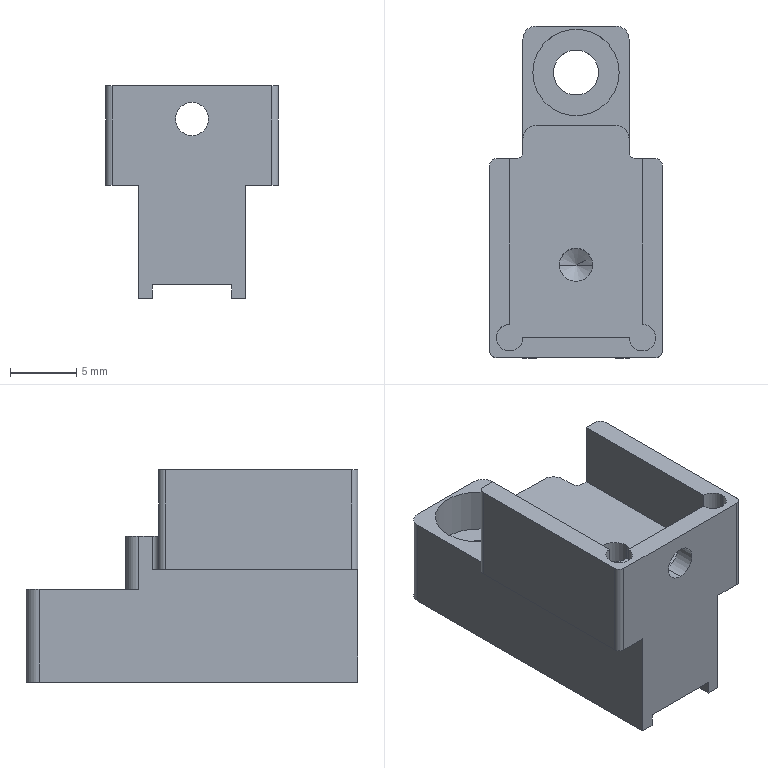Part | SolidWorks | features ICE 9, Fillet 3, HoleWzd 3, Extrusion 1 | 1 solid | 46 faces | box 13 x 25 x 16 mm | volume 2086 mm3 | plane 23 | cylinder 21 | cone 2 | commonest cylinder face diameters 2 x7 1 x6 2.5 x4 3.4 x2 6.5 x2
STEP:
#1=CARTESIAN_POINT('',(5.,-10.,11.));
#2=VERTEX_POINT('',#1);
#3=CARTESIAN_POINT('',(6.,-11.,11.));
#4=VERTEX_POINT('',#3);
#5=CARTESIAN_POINT('',(5.,-11.,11.));
#6=DIRECTION('',(0.,0.,-1.));
#7=DIRECTION('',(1.,0.,0.));
#8=AXIS2_PLACEMENT_3D('',#5,#6,#7);
#9=CIRCLE('',#8,1.);
#10=EDGE_CURVE('',#2,#4,#9,.T.);
#11=ORIENTED_EDGE('',*,*,#10,.T.);
#12=CARTESIAN_POINT('',(6.,-11.,16.));
#13=VERTEX_POINT('',#12);
#14=CARTESIAN_POINT('',(6.,-11.,8.172));
#15=DIRECTION('',(0.,0.,1.));
#16=VECTOR('',#15,1000.);
#17=LINE('',#14,#16);
#18=EDGE_CURVE('',#4,#13,#17,.T.);
#19=ORIENTED_EDGE('',*,*,#18,.T.);
#20=CARTESIAN_POINT('',(5.,-10.,16.));
#21=VERTEX_POINT('',#20);
#22=CARTESIAN_POINT('',(5.,-11.,16.));
#23=DIRECTION('',(0.,0.,1.));
#24=DIRECTION('',(-1.,0.,0.));
#25=AXIS2_PLACEMENT_3D('',#22,#23,#24);
#26=CIRCLE('',#25,1.);
#27=EDGE_CURVE('',#13,#21,#26,.T.);
#28=ORIENTED_EDGE('',*,*,#27,.T.);
#29=CARTESIAN_POINT('',(5.,-10.,8.172));
#30=DIRECTION('',(0.,0.,1.));
#31=VECTOR('',#30,1000.);
#32=LINE('',#29,#31);
#33=EDGE_CURVE('',#2,#21,#32,.T.);
#34=ORIENTED_EDGE('',*,*,#33,.F.);
#35=EDGE_LOOP('',(#11,#19,#28,#34));
#36=FACE_OUTER_BOUND('',#35,.T.);
#37=CARTESIAN_POINT('',(5.,-11.,8.172));
#38=DIRECTION('',(0.,0.,1.));
#39=DIRECTION('',(1.,0.,0.));
#40=AXIS2_PLACEMENT_3D('',#37,#38,#39);
#41=CYLINDRICAL_SURFACE('',#40,1.);
#42=ADVANCED_FACE('',(#36),#41,.F.);
#43=CARTESIAN_POINT('',(0.,-11.,14.75));
#44=VERTEX_POINT('',#43);
#45=CARTESIAN_POINT('',(0.,-11.,12.25));
#46=VERTEX_POINT('',#45);
#47=CARTESIAN_POINT('',(0.,-11.,13.5));
#48=DIRECTION('',(0.,-1.,0.));
#49=DIRECTION('',(1.,0.,0.));
#50=AXIS2_PLACEMENT_3D('',#47,#48,#49);
#51=CIRCLE('',#50,1.25);
#52=EDGE_CURVE('',#44,#46,#51,.T.);
#53=ORIENTED_EDGE('',*,*,#52,.F.);
#54=CARTESIAN_POINT('',(0.,-12.5,14.75));
#55=VERTEX_POINT('',#54);
#56=CARTESIAN_POINT('',(0.,-12.5,14.75));
#57=DIRECTION('',(0.,-1.,0.));
#58=VECTOR('',#57,1000.);
#59=LINE('',#56,#58);
#60=EDGE_CURVE('',#44,#55,#59,.T.);
#61=ORIENTED_EDGE('',*,*,#60,.T.);
#62=CARTESIAN_POINT('',(0.,-12.5,12.25));
#63=VERTEX_POINT('',#62);
#64=CARTESIAN_POINT('',(0.,-12.5,13.5));
#65=DIRECTION('',(0.,-1.,0.));
#66=DIRECTION('',(0.,0.,-1.));
#67=AXIS2_PLACEMENT_3D('',#64,#65,#66);
#68=CIRCLE('',#67,1.25);
#69=EDGE_CURVE('',#55,#63,#68,.T.);
#70=ORIENTED_EDGE('',*,*,#69,.T.);
#71=CARTESIAN_POINT('',(0.,-12.5,12.25));
#72=DIRECTION('',(0.,-1.,0.));
#73=VECTOR('',#72,1000.);
#74=LINE('',#71,#73);
#75=EDGE_CURVE('',#46,#63,#74,.T.);
#76=ORIENTED_EDGE('',*,*,#75,.F.);
#77=EDGE_LOOP('',(#53,#61,#70,#76));
#78=FACE_OUTER_BOUND('',#77,.T.);
#79=CARTESIAN_POINT('',(0.,-12.5,13.5));
#80=DIRECTION('',(0.,-1.,0.));
#81=DIRECTION('',(0.,0.,-1.));
#82=AXIS2_PLACEMENT_3D('',#79,#80,#81);
#83=CYLINDRICAL_SURFACE('',#82,1.25);
#84=ADVANCED_FACE('',(#78),#83,.F.);
#85=CARTESIAN_POINT('',(-1.25,-5.5,3.5));
#86=VERTEX_POINT('',#85);
#87=CARTESIAN_POINT('',(1.25,-5.5,3.5));
#88=VERTEX_POINT('',#87);
#89=CARTESIAN_POINT('',(0.,-5.5,3.5));
#90=DIRECTION('',(0.,0.,1.));
#91=DIRECTION('',(1.,0.,0.));
#92=AXIS2_PLACEMENT_3D('',#89,#90,#91);
#93=CIRCLE('',#92,1.25);
#94=EDGE_CURVE('',#86,#88,#93,.T.);
#95=ORIENTED_EDGE('',*,*,#94,.F.);
#96=CARTESIAN_POINT('',(-1.25,-5.5,11.));
#97=VERTEX_POINT('',#96);
#98=CARTESIAN_POINT('',(-1.25,-5.5,11.));
#99=DIRECTION('',(0.,0.,1.));
#100=VECTOR('',#99,1000.);
#101=LINE('',#98,#100);
#102=EDGE_CURVE('',#86,#97,#101,.T.);
#103=ORIENTED_EDGE('',*,*,#102,.T.);
#104=CARTESIAN_POINT('',(1.25,-5.5,11.));
#105=VERTEX_POINT('',#104);
#106=CARTESIAN_POINT('',(0.,-5.5,11.));
#107=DIRECTION('',(0.,0.,1.));
#108=DIRECTION('',(1.,0.,0.));
#109=AXIS2_PLACEMENT_3D('',#106,#107,#108);
#110=CIRCLE('',#109,1.25);
#111=EDGE_CURVE('',#97,#105,#110,.T.);
#112=ORIENTED_EDGE('',*,*,#111,.T.);
#113=CARTESIAN_POINT('',(1.25,-5.5,11.));
#114=DIRECTION('',(0.,0.,1.));
#115=VECTOR('',#114,1000.);
#116=LINE('',#113,#115);
#117=EDGE_CURVE('',#88,#105,#116,.T.);
#118=ORIENTED_EDGE('',*,*,#117,.F.);
#119=EDGE_LOOP('',(#95,#103,#112,#118));
#120=FACE_OUTER_BOUND('',#119,.T.);
#121=CARTESIAN_POINT('',(0.,-5.5,11.));
#122=DIRECTION('',(0.,0.,1.));
#123=DIRECTION('',(1.,0.,0.));
#124=AXIS2_PLACEMENT_3D('',#121,#122,#123);
#125=CYLINDRICAL_SURFACE('',#124,1.25);
#126=ADVANCED_FACE('',(#120),#125,.F.);
#127=CARTESIAN_POINT('',(0.,-5.5,2.749));
#128=VERTEX_POINT('',#127);
#129=CARTESIAN_POINT('',(1.25,-5.5,3.5));
#130=DIRECTION('',(0.8572,0.,0.515));
#131=VECTOR('',#130,1000.);
#132=LINE('',#129,#131);
#133=EDGE_CURVE('',#128,#88,#132,.T.);
#134=ORIENTED_EDGE('',*,*,#133,.F.);
#135=CARTESIAN_POINT('',(-1.25,-5.5,3.5));
#136=DIRECTION('',(-0.8572,0.,0.515));
#137=VECTOR('',#136,1000.);
#138=LINE('',#135,#137);
#139=EDGE_CURVE('',#128,#86,#138,.T.);
#140=ORIENTED_EDGE('',*,*,#139,.T.);
#141=ORIENTED_EDGE('',*,*,#94,.T.);
#142=EDGE_LOOP('',(#134,#140,#141));
#143=FACE_OUTER_BOUND('',#142,.T.);
#144=CARTESIAN_POINT('',(0.,-5.5,3.5));
#145=DIRECTION('',(0.,0.,1.));
#146=DIRECTION('',(1.,0.,0.));
#147=AXIS2_PLACEMENT_3D('',#144,#145,#146);
#148=CONICAL_SURFACE('',#147,1.25,1.03);
#149=ADVANCED_FACE('',(#143),#148,.F.);
#150=CARTESIAN_POINT('',(-3.25,9.,3.6));
#151=VERTEX_POINT('',#150);
#152=CARTESIAN_POINT('',(3.25,9.,3.6));
#153=VERTEX_POINT('',#152);
#154=CARTESIAN_POINT('',(0.,9.,3.6));
#155=DIRECTION('',(0.,0.,1.));
#156=DIRECTION('',(1.,0.,0.));
#157=AXIS2_PLACEMENT_3D('',#154,#155,#156);
#158=CIRCLE('',#157,3.25);
#159=EDGE_CURVE('',#151,#153,#158,.T.);
#160=ORIENTED_EDGE('',*,*,#159,.F.);
#161=CARTESIAN_POINT('',(-3.25,9.,7.));
#162=VERTEX_POINT('',#161);
#163=CARTESIAN_POINT('',(-3.25,9.,9.));
#164=DIRECTION('',(0.,0.,1.));
#165=VECTOR('',#164,1000.);
#166=LINE('',#163,#165);
#167=EDGE_CURVE('',#151,#162,#166,.T.);
#168=ORIENTED_EDGE('',*,*,#167,.T.);
#169=CARTESIAN_POINT('',(3.25,9.,7.));
#170=VERTEX_POINT('',#169);
#171=CARTESIAN_POINT('',(0.,9.,7.));
#172=DIRECTION('',(0.,0.,1.));
#173=DIRECTION('',(1.,0.,0.));
#174=AXIS2_PLACEMENT_3D('',#171,#172,#173);
#175=CIRCLE('',#174,3.25);
#176=EDGE_CURVE('',#162,#170,#175,.T.);
#177=ORIENTED_EDGE('',*,*,#176,.T.);
#178=CARTESIAN_POINT('',(3.25,9.,9.));
#179=DIRECTION('',(0.,0.,1.));
#180=VECTOR('',#179,1000.);
#181=LINE('',#178,#180);
#182=EDGE_CURVE('',#153,#170,#181,.T.);
#183=ORIENTED_EDGE('',*,*,#182,.F.);
#184=EDGE_LOOP('',(#160,#168,#177,#183));
#185=FACE_OUTER_BOUND('',#184,.T.);
#186=CARTESIAN_POINT('',(0.,9.,9.));
#187=DIRECTION('',(0.,0.,1.));
#188=DIRECTION('',(1.,0.,0.));
#189=AXIS2_PLACEMENT_3D('',#186,#187,#188);
#190=CYLINDRICAL_SURFACE('',#189,3.25);
#191=ADVANCED_FACE('',(#185),#190,.F.);
#192=CARTESIAN_POINT('',(-1.7,9.,1.));
#193=VERTEX_POINT('',#192);
#194=CARTESIAN_POINT('',(1.7,9.,1.));
#195=VERTEX_POINT('',#194);
#196=CARTESIAN_POINT('',(0.,9.,1.));
#197=DIRECTION('',(0.,0.,1.));
#198=DIRECTION('',(1.,0.,0.));
#199=AXIS2_PLACEMENT_3D('',#196,#197,#198);
#200=CIRCLE('',#199,1.7);
#201=EDGE_CURVE('',#193,#195,#200,.T.);
#202=ORIENTED_EDGE('',*,*,#201,.F.);
#203=CARTESIAN_POINT('',(-1.7,9.,3.6));
#204=VERTEX_POINT('',#203);
#205=CARTESIAN_POINT('',(-1.7,9.,9.));
#206=DIRECTION('',(0.,0.,1.));
#207=VECTOR('',#206,1000.);
#208=LINE('',#205,#207);
#209=EDGE_CURVE('',#193,#204,#208,.T.);
#210=ORIENTED_EDGE('',*,*,#209,.T.);
#211=CARTESIAN_POINT('',(1.7,9.,3.6));
#212=VERTEX_POINT('',#211);
#213=CARTESIAN_POINT('',(0.,9.,3.6));
#214=DIRECTION('',(0.,0.,1.));
#215=DIRECTION('',(1.,0.,0.));
#216=AXIS2_PLACEMENT_3D('',#213,#214,#215);
#217=CIRCLE('',#216,1.7);
#218=EDGE_CURVE('',#204,#212,#217,.T.);
#219=ORIENTED_EDGE('',*,*,#218,.T.);
#220=CARTESIAN_POINT('',(1.7,9.,9.));
#221=DIRECTION('',(0.,0.,1.));
#222=VECTOR('',#221,1000.);
#223=LINE('',#220,#222);
#224=EDGE_CURVE('',#195,#212,#223,.T.);
#225=ORIENTED_EDGE('',*,*,#224,.F.);
#226=EDGE_LOOP('',(#202,#210,#219,#225));
#227=FACE_OUTER_BOUND('',#226,.T.);
#228=CARTESIAN_POINT('',(0.,9.,9.));
#229=DIRECTION('',(0.,0.,1.));
#230=DIRECTION('',(1.,0.,0.));
#231=AXIS2_PLACEMENT_3D('',#228,#229,#230);
#232=CYLINDRICAL_SURFACE('',#231,1.7);
#233=ADVANCED_FACE('',(#227),#232,.F.);
#234=CARTESIAN_POINT('',(3.,12.5,7.));
#235=VERTEX_POINT('',#234);
#236=CARTESIAN_POINT('',(-3.,12.5,7.));
#237=VERTEX_POINT('',#236);
#238=CARTESIAN_POINT('',(-6.5,12.5,7.));
#239=DIRECTION('',(-1.,0.,0.));
#240=VECTOR('',#239,1000.);
#241=LINE('',#238,#240);
#242=EDGE_CURVE('',#235,#237,#241,.T.);
#243=ORIENTED_EDGE('',*,*,#242,.F.);
#244=CARTESIAN_POINT('',(3.,12.5,1.));
#245=VERTEX_POINT('',#244);
#246=CARTESIAN_POINT('',(3.,12.5,10.));
#247=DIRECTION('',(0.,0.,-1.));
#248=VECTOR('',#247,1000.);
#249=LINE('',#246,#248);
#250=EDGE_CURVE('',#235,#245,#249,.T.);
#251=ORIENTED_EDGE('',*,*,#250,.T.);
#252=CARTESIAN_POINT('',(-3.,12.5,1.));
#253=VERTEX_POINT('',#252);
#254=CARTESIAN_POINT('',(3.,12.5,1.));
#255=DIRECTION('',(1.,0.,0.));
#256=VECTOR('',#255,1000.);
#257=LINE('',#254,#256);
#258=EDGE_CURVE('',#253,#245,#257,.T.);
#259=ORIENTED_EDGE('',*,*,#258,.F.);
#260=CARTESIAN_POINT('',(-3.,12.5,10.));
#261=DIRECTION('',(0.,0.,1.));
#262=VECTOR('',#261,1000.);
#263=LINE('',#260,#262);
#264=EDGE_CURVE('',#253,#237,#263,.T.);
#265=ORIENTED_EDGE('',*,*,#264,.T.);
#266=EDGE_LOOP('',(#243,#251,#259,#265));
#267=FACE_OUTER_BOUND('',#266,.T.);
#268=CARTESIAN_POINT('',(-6.5,12.5,10.));
#269=DIRECTION('',(0.,-1.,0.));
#270=DIRECTION('',(0.,0.,-1.));
#271=AXIS2_PLACEMENT_3D('',#268,#269,#270);
#272=PLANE('',#271);
#273=ADVANCED_FACE('',(#267),#272,.F.);
#274=ORIENTED_EDGE('',*,*,#250,.F.);
#275=CARTESIAN_POINT('',(4.,11.5,7.));
#276=VERTEX_POINT('',#275);
#277=CARTESIAN_POINT('',(3.,11.5,7.));
#278=DIRECTION('',(0.,0.,-1.));
#279=DIRECTION('',(1.,0.,0.));
#280=AXIS2_PLACEMENT_3D('',#277,#278,#279);
#281=CIRCLE('',#280,1.);
#282=EDGE_CURVE('',#235,#276,#281,.T.);
#283=ORIENTED_EDGE('',*,*,#282,.T.);
#284=CARTESIAN_POINT('',(4.,11.5,0.));
#285=VERTEX_POINT('',#284);
#286=CARTESIAN_POINT('',(4.,11.5,0.));
#287=DIRECTION('',(0.,0.,1.));
#288=VECTOR('',#287,1000.);
#289=LINE('',#286,#288);
#290=EDGE_CURVE('',#285,#276,#289,.T.);
#291=ORIENTED_EDGE('',*,*,#290,.F.);
#292=CARTESIAN_POINT('',(3.,12.5,0.));
#293=VERTEX_POINT('',#292);
#294=CARTESIAN_POINT('',(3.,11.5,0.));
#295=DIRECTION('',(0.,0.,-1.));
#296=DIRECTION('',(1.,0.,0.));
#297=AXIS2_PLACEMENT_3D('',#294,#295,#296);
#298=CIRCLE('',#297,1.);
#299=EDGE_CURVE('',#293,#285,#298,.T.);
#300=ORIENTED_EDGE('',*,*,#299,.F.);
#301=CARTESIAN_POINT('',(3.,12.5,1.));
#302=DIRECTION('',(0.,0.,-1.));
#303=VECTOR('',#302,1000.);
#304=LINE('',#301,#303);
#305=EDGE_CURVE('',#245,#293,#304,.T.);
#306=ORIENTED_EDGE('',*,*,#305,.F.);
#307=EDGE_LOOP('',(#274,#283,#291,#300,#306));
#308=FACE_OUTER_BOUND('',#307,.T.);
#309=CARTESIAN_POINT('',(3.,11.5,0.));
#310=DIRECTION('',(0.,0.,1.));
#311=DIRECTION('',(1.,0.,0.));
#312=AXIS2_PLACEMENT_3D('',#309,#310,#311);
#313=CYLINDRICAL_SURFACE('',#312,1.);
#314=ADVANCED_FACE('',(#308),#313,.T.);
#315=CARTESIAN_POINT('',(-4.,11.5,7.));
#316=VERTEX_POINT('',#315);
#317=CARTESIAN_POINT('',(-4.,11.5,0.));
#318=VERTEX_POINT('',#317);
#319=CARTESIAN_POINT('',(-4.,11.5,0.));
#320=DIRECTION('',(0.,0.,-1.));
#321=VECTOR('',#320,1000.);
#322=LINE('',#319,#321);
#323=EDGE_CURVE('',#316,#318,#322,.T.);
#324=ORIENTED_EDGE('',*,*,#323,.F.);
#325=CARTESIAN_POINT('',(-3.,11.5,7.));
#326=DIRECTION('',(0.,0.,-1.));
#327=DIRECTION('',(1.,0.,0.));
#328=AXIS2_PLACEMENT_3D('',#325,#326,#327);
#329=CIRCLE('',#328,1.);
#330=EDGE_CURVE('',#316,#237,#329,.T.);
#331=ORIENTED_EDGE('',*,*,#330,.T.);
#332=ORIENTED_EDGE('',*,*,#264,.F.);
#333=CARTESIAN_POINT('',(-3.,12.5,0.));
#334=VERTEX_POINT('',#333);
#335=CARTESIAN_POINT('',(-3.,12.5,10.));
#336=DIRECTION('',(0.,0.,1.));
#337=VECTOR('',#336,1000.);
#338=LINE('',#335,#337);
#339=EDGE_CURVE('',#334,#253,#338,.T.);
#340=ORIENTED_EDGE('',*,*,#339,.F.);
#341=CARTESIAN_POINT('',(-3.,11.5,0.));
#342=DIRECTION('',(0.,0.,-1.));
#343=DIRECTION('',(1.,0.,0.));
#344=AXIS2_PLACEMENT_3D('',#341,#342,#343);
#345=CIRCLE('',#344,1.);
#346=EDGE_CURVE('',#318,#334,#345,.T.);
#347=ORIENTED_EDGE('',*,*,#346,.F.);
#348=EDGE_LOOP('',(#324,#331,#332,#340,#347));
#349=FACE_OUTER_BOUND('',#348,.T.);
#350=CARTESIAN_POINT('',(-3.,11.5,10.));
#351=DIRECTION('',(0.,0.,1.));
#352=DIRECTION('',(1.,0.,0.));
#353=AXIS2_PLACEMENT_3D('',#350,#351,#352);
#354=CYLINDRICAL_SURFACE('',#353,1.);
#355=ADVANCED_FACE('',(#349),#354,.T.);
#356=CARTESIAN_POINT('',(4.,-12.5,0.));
#357=VERTEX_POINT('',#356);
#358=CARTESIAN_POINT('',(4.,-12.5,8.5));
#359=VERTEX_POINT('',#358);
#360=CARTESIAN_POINT('',(4.,-12.5,10.));
#361=DIRECTION('',(0.,0.,1.));
#362=VECTOR('',#361,1000.);
#363=LINE('',#360,#362);
#364=EDGE_CURVE('',#357,#359,#363,.T.);
#365=ORIENTED_EDGE('',*,*,#364,.F.);
#366=CARTESIAN_POINT('',(4.,12.5,0.));
#367=DIRECTION('',(0.,-1.,0.));
#368=VECTOR('',#367,1000.);
#369=LINE('',#366,#368);
#370=EDGE_CURVE('',#285,#357,#369,.T.);
#371=ORIENTED_EDGE('',*,*,#370,.F.);
#372=ORIENTED_EDGE('',*,*,#290,.T.);
#373=CARTESIAN_POINT('',(4.,4.,7.));
#374=VERTEX_POINT('',#373);
#375=CARTESIAN_POINT('',(4.,12.5,7.));
#376=DIRECTION('',(0.,1.,0.));
#377=VECTOR('',#376,1000.);
#378=LINE('',#375,#377);
#379=EDGE_CURVE('',#374,#276,#378,.T.);
#380=ORIENTED_EDGE('',*,*,#379,.F.);
#381=CARTESIAN_POINT('',(4.,4.,11.));
#382=VERTEX_POINT('',#381);
#383=CARTESIAN_POINT('',(4.,4.,0.));
#384=DIRECTION('',(0.,0.,1.));
#385=VECTOR('',#384,1000.);
#386=LINE('',#383,#385);
#387=EDGE_CURVE('',#374,#382,#386,.T.);
#388=ORIENTED_EDGE('',*,*,#387,.T.);
#389=CARTESIAN_POINT('',(4.,3.,11.));
#390=VERTEX_POINT('',#389);
#391=CARTESIAN_POINT('',(4.,3.,11.));
#392=DIRECTION('',(0.,1.,0.));
#393=VECTOR('',#392,1000.);
#394=LINE('',#391,#393);
#395=EDGE_CURVE('',#390,#382,#394,.T.);
#396=ORIENTED_EDGE('',*,*,#395,.F.);
#397=CARTESIAN_POINT('',(4.,3.,8.5));
#398=VERTEX_POINT('',#397);
#399=CARTESIAN_POINT('',(4.,3.,0.));
#400=DIRECTION('',(0.,0.,-1.));
#401=VECTOR('',#400,1000.);
#402=LINE('',#399,#401);
#403=EDGE_CURVE('',#390,#398,#402,.T.);
#404=ORIENTED_EDGE('',*,*,#403,.T.);
#405=CARTESIAN_POINT('',(4.,-16.236,8.5));
#406=DIRECTION('',(0.,-1.,0.));
#407=VECTOR('',#406,1000.);
#408=LINE('',#405,#407);
#409=EDGE_CURVE('',#398,#359,#408,.T.);
#410=ORIENTED_EDGE('',*,*,#409,.T.);
#411=EDGE_LOOP('',(#365,#371,#372,#380,#388,#396,#404,#410));
#412=FACE_OUTER_BOUND('',#411,.T.);
#413=CARTESIAN_POINT('',(4.,12.5,0.));
#414=DIRECTION('',(-1.,0.,0.));
#415=DIRECTION('',(0.,-1.,0.));
#416=AXIS2_PLACEMENT_3D('',#413,#414,#415);
#417=PLANE('',#416);
#418=ADVANCED_FACE('',(#412),#417,.F.);
#419=CARTESIAN_POINT('',(-4.,-12.5,8.5));
#420=VERTEX_POINT('',#419);
#421=CARTESIAN_POINT('',(-4.,3.,8.5));
#422=VERTEX_POINT('',#421);
#423=CARTESIAN_POINT('',(-4.,3.5,8.5));
#424=DIRECTION('',(0.,1.,0.));
#425=VECTOR('',#424,1000.);
#426=LINE('',#423,#425);
#427=EDGE_CURVE('',#420,#422,#426,.T.);
#428=ORIENTED_EDGE('',*,*,#427,.T.);
#429=CARTESIAN_POINT('',(-4.,3.,11.));
#430=VERTEX_POINT('',#429);
#431=CARTESIAN_POINT('',(-4.,3.,10.));
#432=DIRECTION('',(0.,0.,1.));
#433=VECTOR('',#432,1000.);
#434=LINE('',#431,#433);
#435=EDGE_CURVE('',#422,#430,#434,.T.);
#436=ORIENTED_EDGE('',*,*,#435,.T.);
#437=CARTESIAN_POINT('',(-4.,4.,11.));
#438=VERTEX_POINT('',#437);
#439=CARTESIAN_POINT('',(-4.,4.,11.));
#440=DIRECTION('',(0.,-1.,0.));
#441=VECTOR('',#440,1000.);
#442=LINE('',#439,#441);
#443=EDGE_CURVE('',#438,#430,#442,.T.);
#444=ORIENTED_EDGE('',*,*,#443,.F.);
#445=CARTESIAN_POINT('',(-4.,4.,7.));
#446=VERTEX_POINT('',#445);
#447=CARTESIAN_POINT('',(-4.,4.,0.));
#448=DIRECTION('',(0.,0.,-1.));
#449=VECTOR('',#448,1000.);
#450=LINE('',#447,#449);
#451=EDGE_CURVE('',#438,#446,#450,.T.);
#452=ORIENTED_EDGE('',*,*,#451,.T.);
#453=CARTESIAN_POINT('',(-4.,12.5,7.));
#454=DIRECTION('',(0.,-1.,0.));
#455=VECTOR('',#454,1000.);
#456=LINE('',#453,#455);
#457=EDGE_CURVE('',#316,#446,#456,.T.);
#458=ORIENTED_EDGE('',*,*,#457,.F.);
#459=ORIENTED_EDGE('',*,*,#323,.T.);
#460=CARTESIAN_POINT('',(-4.,-12.5,0.));
#461=VERTEX_POINT('',#460);
#462=CARTESIAN_POINT('',(-4.,12.5,0.));
#463=DIRECTION('',(0.,1.,0.));
#464=VECTOR('',#463,1000.);
#465=LINE('',#462,#464);
#466=EDGE_CURVE('',#461,#318,#465,.T.);
#467=ORIENTED_EDGE('',*,*,#466,.F.);
#468=CARTESIAN_POINT('',(-4.,-12.5,10.));
#469=DIRECTION('',(0.,0.,-1.));
#470=VECTOR('',#469,1000.);
#471=LINE('',#468,#470);
#472=EDGE_CURVE('',#420,#461,#471,.T.);
#473=ORIENTED_EDGE('',*,*,#472,.F.);
#474=EDGE_LOOP('',(#428,#436,#444,#452,#458,#459,#467,#473));
#475=FACE_OUTER_BOUND('',#474,.T.);
#476=CARTESIAN_POINT('',(-4.,12.5,0.));
#477=DIRECTION('',(1.,0.,0.));
#478=DIRECTION('',(0.,1.,0.));
#479=AXIS2_PLACEMENT_3D('',#476,#477,#478);
#480=PLANE('',#479);
#481=ADVANCED_FACE('',(#475),#480,.F.);
#482=CARTESIAN_POINT('',(4.5,2.5,8.5));
#483=VERTEX_POINT('',#482);
#484=CARTESIAN_POINT('',(4.5,2.5,11.));
#485=VERTEX_POINT('',#484);
#486=CARTESIAN_POINT('',(4.5,2.5,10.));
#487=DIRECTION('',(0.,0.,1.));
#488=VECTOR('',#487,1000.);
#489=LINE('',#486,#488);
#490=EDGE_CURVE('',#483,#485,#489,.T.);
#491=ORIENTED_EDGE('',*,*,#490,.F.);
#492=CARTESIAN_POINT('',(4.5,3.,8.5));
#493=DIRECTION('',(0.,0.,-1.));
#494=DIRECTION('',(1.,0.,0.));
#495=AXIS2_PLACEMENT_3D('',#492,#493,#494);
#496=CIRCLE('',#495,0.5);
#497=EDGE_CURVE('',#483,#398,#496,.T.);
#498=ORIENTED_EDGE('',*,*,#497,.T.);
#499=ORIENTED_EDGE('',*,*,#403,.F.);
#500=CARTESIAN_POINT('',(4.5,3.,11.));
#501=DIRECTION('',(0.,0.,-1.));
#502=DIRECTION('',(1.,0.,0.));
#503=AXIS2_PLACEMENT_3D('',#500,#501,#502);
#504=CIRCLE('',#503,0.5);
#505=EDGE_CURVE('',#485,#390,#504,.T.);
#506=ORIENTED_EDGE('',*,*,#505,.F.);
#507=EDGE_LOOP('',(#491,#498,#499,#506));
#508=FACE_OUTER_BOUND('',#507,.T.);
#509=CARTESIAN_POINT('',(4.5,3.,0.));
#510=DIRECTION('',(0.,0.,-1.));
#511=DIRECTION('',(-1.,0.,0.));
#512=AXIS2_PLACEMENT_3D('',#509,#510,#511);
#513=CYLINDRICAL_SURFACE('',#512,0.5);
#514=ADVANCED_FACE('',(#508),#513,.F.);
#515=ORIENTED_EDGE('',*,*,#435,.F.);
#516=CARTESIAN_POINT('',(-4.5,2.5,8.5));
#517=VERTEX_POINT('',#516);
#518=CARTESIAN_POINT('',(-4.5,3.,8.5));
#519=DIRECTION('',(0.,0.,-1.));
#520=DIRECTION('',(0.,-1.,0.));
#521=AXIS2_PLACEMENT_3D('',#518,#519,#520);
#522=CIRCLE('',#521,0.5);
#523=EDGE_CURVE('',#422,#517,#522,.T.);
#524=ORIENTED_EDGE('',*,*,#523,.T.);
#525=CARTESIAN_POINT('',(-4.5,2.5,11.));
#526=VERTEX_POINT('',#525);
#527=CARTESIAN_POINT('',(-4.5,2.5,0.));
#528=DIRECTION('',(0.,0.,-1.));
#529=VECTOR('',#528,1000.);
#530=LINE('',#527,#529);
#531=EDGE_CURVE('',#526,#517,#530,.T.);
#532=ORIENTED_EDGE('',*,*,#531,.F.);
#533=CARTESIAN_POINT('',(-4.5,3.,11.));
#534=DIRECTION('',(0.,0.,-1.));
#535=DIRECTION('',(1.,0.,0.));
#536=AXIS2_PLACEMENT_3D('',#533,#534,#535);
#537=CIRCLE('',#536,0.5);
#538=EDGE_CURVE('',#430,#526,#537,.T.);
#539=ORIENTED_EDGE('',*,*,#538,.F.);
#540=EDGE_LOOP('',(#515,#524,#532,#539));
#541=FACE_OUTER_BOUND('',#540,.T.);
#542=CARTESIAN_POINT('',(-4.5,3.,0.));
#543=DIRECTION('',(0.,0.,-1.));
#544=DIRECTION('',(-1.,0.,0.));
#545=AXIS2_PLACEMENT_3D('',#542,#543,#544);
#546=CYLINDRICAL_SURFACE('',#545,0.5);
#547=ADVANCED_FACE('',(#541),#546,.F.);
#548=CARTESIAN_POINT('',(-3.,-12.5,0.));
#549=VERTEX_POINT('',#548);
#550=CARTESIAN_POINT('',(-6.5,-12.5,0.));
#551=DIRECTION('',(1.,0.,0.));
#552=VECTOR('',#551,1000.);
#553=LINE('',#550,#552);
#554=EDGE_CURVE('',#461,#549,#553,.T.);
#555=ORIENTED_EDGE('',*,*,#554,.F.);
#556=ORIENTED_EDGE('',*,*,#466,.T.);
#557=ORIENTED_EDGE('',*,*,#346,.T.);
#558=CARTESIAN_POINT('',(-3.,-20.089,0.));
#559=DIRECTION('',(0.,1.,0.));
#560=VECTOR('',#559,1000.);
#561=LINE('',#558,#560);
#562=EDGE_CURVE('',#549,#334,#561,.T.);
#563=ORIENTED_EDGE('',*,*,#562,.F.);
#564=EDGE_LOOP('',(#555,#556,#557,#563));
#565=FACE_OUTER_BOUND('',#564,.T.);
#566=CARTESIAN_POINT('',(0.,0.,0.));
#567=DIRECTION('',(0.,0.,1.));
#568=DIRECTION('',(1.,0.,0.));
#569=AXIS2_PLACEMENT_3D('',#566,#567,#568);
#570=PLANE('',#569);
#571=ADVANCED_FACE('',(#565),#570,.F.);
#572=CARTESIAN_POINT('',(6.5,-12.,16.));
#573=VERTEX_POINT('',#572);
#574=CARTESIAN_POINT('',(6.5,-12.,8.5));
#575=VERTEX_POINT('',#574);
#576=CARTESIAN_POINT('',(6.5,-12.,10.));
#577=DIRECTION('',(0.,0.,-1.));
#578=VECTOR('',#577,1000.);
#579=LINE('',#576,#578);
#580=EDGE_CURVE('',#573,#575,#579,.T.);
#581=ORIENTED_EDGE('',*,*,#580,.T.);
#582=CARTESIAN_POINT('',(6.5,2.,8.5));
#583=VERTEX_POINT('',#582);
#584=CARTESIAN_POINT('',(6.5,-16.236,8.5));
#585=DIRECTION('',(0.,-1.,0.));
#586=VECTOR('',#585,1000.);
#587=LINE('',#584,#586);
#588=EDGE_CURVE('',#583,#575,#587,.T.);
#589=ORIENTED_EDGE('',*,*,#588,.F.);
#590=CARTESIAN_POINT('',(6.5,2.,16.));
#591=VERTEX_POINT('',#590);
#592=CARTESIAN_POINT('',(6.5,2.,10.));
#593=DIRECTION('',(0.,0.,1.));
#594=VECTOR('',#593,1000.);
#595=LINE('',#592,#594);
#596=EDGE_CURVE('',#583,#591,#595,.T.);
#597=ORIENTED_EDGE('',*,*,#596,.T.);
#598=CARTESIAN_POINT('',(6.5,-12.,16.));
#599=DIRECTION('',(0.,1.,0.));
#600=VECTOR('',#599,1000.);
#601=LINE('',#598,#600);
#602=EDGE_CURVE('',#573,#591,#601,.T.);
#603=ORIENTED_EDGE('',*,*,#602,.F.);
#604=EDGE_LOOP('',(#581,#589,#597,#603));
#605=FACE_OUTER_BOUND('',#604,.T.);
#606=CARTESIAN_POINT('',(6.5,12.5,10.));
#607=DIRECTION('',(-1.,0.,0.));
#608=DIRECTION('',(0.,-1.,0.));
#609=AXIS2_PLACEMENT_3D('',#606,#607,#608);
#610=PLANE('',#609);
#611=ADVANCED_FACE('',(#605),#610,.F.);
#612=CARTESIAN_POINT('',(-6.5,2.,16.));
#613=VERTEX_POINT('',#612);
#614=CARTESIAN_POINT('',(-6.5,2.,8.5));
#615=VERTEX_POINT('',#614);
#616=CARTESIAN_POINT('',(-6.5,2.,10.));
#617=DIRECTION('',(0.,0.,-1.));
#618=VECTOR('',#617,1000.);
#619=LINE('',#616,#618);
#620=EDGE_CURVE('',#613,#615,#619,.T.);
#621=ORIENTED_EDGE('',*,*,#620,.T.);
#622=CARTESIAN_POINT('',(-6.5,-12.,8.5));
#623=VERTEX_POINT('',#622);
#624=CARTESIAN_POINT('',(-6.5,3.5,8.5));
#625=DIRECTION('',(0.,1.,0.));
#626=VECTOR('',#625,1000.);
#627=LINE('',#624,#626);
#628=EDGE_CURVE('',#623,#615,#627,.T.);
#629=ORIENTED_EDGE('',*,*,#628,.F.);
#630=CARTESIAN_POINT('',(-6.5,-12.,16.));
#631=VERTEX_POINT('',#630);
#632=CARTESIAN_POINT('',(-6.5,-12.,10.));
#633=DIRECTION('',(0.,0.,1.));
#634=VECTOR('',#633,1000.);
#635=LINE('',#632,#634);
#636=EDGE_CURVE('',#623,#631,#635,.T.);
#637=ORIENTED_EDGE('',*,*,#636,.T.);
#638=CARTESIAN_POINT('',(-6.5,2.,16.));
#639=DIRECTION('',(0.,-1.,0.));
#640=VECTOR('',#639,1000.);
#641=LINE('',#638,#640);
#642=EDGE_CURVE('',#613,#631,#641,.T.);
#643=ORIENTED_EDGE('',*,*,#642,.F.);
#644=EDGE_LOOP('',(#621,#629,#637,#643));
#645=FACE_OUTER_BOUND('',#644,.T.);
#646=CARTESIAN_POINT('',(-6.5,12.5,10.));
#647=DIRECTION('',(1.,0.,0.));
#648=DIRECTION('',(0.,1.,0.));
#649=AXIS2_PLACEMENT_3D('',#646,#647,#648);
#650=PLANE('',#649);
#651=ADVANCED_FACE('',(#645),#650,.F.);
#652=CARTESIAN_POINT('',(0.,-12.5,13.5));
#653=DIRECTION('',(0.,-1.,0.));
#654=DIRECTION('',(0.,0.,-1.));
#655=AXIS2_PLACEMENT_3D('',#652,#653,#654);
#656=CIRCLE('',#655,1.25);
#657=EDGE_CURVE('',#63,#55,#656,.T.);
#658=ORIENTED_EDGE('',*,*,#657,.F.);
#659=ORIENTED_EDGE('',*,*,#69,.F.);
#660=EDGE_LOOP('',(#658,#659));
#661=FACE_BOUND('',#660,.T.);
#662=CARTESIAN_POINT('',(3.,-12.5,0.));
#663=VERTEX_POINT('',#662);
#664=CARTESIAN_POINT('',(-6.5,-12.5,0.));
#665=DIRECTION('',(1.,0.,0.));
#666=VECTOR('',#665,1000.);
#667=LINE('',#664,#666);
#668=EDGE_CURVE('',#663,#357,#667,.T.);
#669=ORIENTED_EDGE('',*,*,#668,.T.);
#670=ORIENTED_EDGE('',*,*,#364,.T.);
#671=CARTESIAN_POINT('',(6.,-12.5,8.5));
#672=VERTEX_POINT('',#671);
#673=CARTESIAN_POINT('',(-6.5,-12.5,8.5));
#674=DIRECTION('',(1.,0.,0.));
#675=VECTOR('',#674,1000.);
#676=LINE('',#673,#675);
#677=EDGE_CURVE('',#359,#672,#676,.T.);
#678=ORIENTED_EDGE('',*,*,#677,.T.);
#679=CARTESIAN_POINT('',(6.,-12.5,16.));
#680=VERTEX_POINT('',#679);
#681=CARTESIAN_POINT('',(6.,-12.5,10.));
#682=DIRECTION('',(0.,0.,1.));
#683=VECTOR('',#682,1000.);
#684=LINE('',#681,#683);
#685=EDGE_CURVE('',#672,#680,#684,.T.);
#686=ORIENTED_EDGE('',*,*,#685,.T.);
#687=CARTESIAN_POINT('',(-6.,-12.5,16.));
#688=VERTEX_POINT('',#687);
#689=CARTESIAN_POINT('',(-6.,-12.5,16.));
#690=DIRECTION('',(1.,0.,0.));
#691=VECTOR('',#690,1000.);
#692=LINE('',#689,#691);
#693=EDGE_CURVE('',#688,#680,#692,.T.);
#694=ORIENTED_EDGE('',*,*,#693,.F.);
#695=CARTESIAN_POINT('',(-6.,-12.5,8.5));
#696=VERTEX_POINT('',#695);
#697=CARTESIAN_POINT('',(-6.,-12.5,10.));
#698=DIRECTION('',(0.,0.,-1.));
#699=VECTOR('',#698,1000.);
#700=LINE('',#697,#699);
#701=EDGE_CURVE('',#688,#696,#700,.T.);
#702=ORIENTED_EDGE('',*,*,#701,.T.);
#703=CARTESIAN_POINT('',(-6.5,-12.5,8.5));
#704=DIRECTION('',(1.,0.,0.));
#705=VECTOR('',#704,1000.);
#706=LINE('',#703,#705);
#707=EDGE_CURVE('',#696,#420,#706,.T.);
#708=ORIENTED_EDGE('',*,*,#707,.T.);
#709=ORIENTED_EDGE('',*,*,#472,.T.);
#710=ORIENTED_EDGE('',*,*,#554,.T.);
#711=CARTESIAN_POINT('',(-3.,-12.5,1.));
#712=VERTEX_POINT('',#711);
#713=CARTESIAN_POINT('',(-3.,-12.5,10.));
#714=DIRECTION('',(0.,0.,1.));
#715=VECTOR('',#714,1000.);
#716=LINE('',#713,#715);
#717=EDGE_CURVE('',#549,#712,#716,.T.);
#718=ORIENTED_EDGE('',*,*,#717,.T.);
#719=CARTESIAN_POINT('',(3.,-12.5,1.));
#720=VERTEX_POINT('',#719);
#721=CARTESIAN_POINT('',(-6.5,-12.5,1.));
#722=DIRECTION('',(1.,0.,0.));
#723=VECTOR('',#722,1000.);
#724=LINE('',#721,#723);
#725=EDGE_CURVE('',#712,#720,#724,.T.);
#726=ORIENTED_EDGE('',*,*,#725,.T.);
#727=CARTESIAN_POINT('',(3.,-12.5,10.));
#728=DIRECTION('',(0.,0.,-1.));
#729=VECTOR('',#728,1000.);
#730=LINE('',#727,#729);
#731=EDGE_CURVE('',#720,#663,#730,.T.);
#732=ORIENTED_EDGE('',*,*,#731,.T.);
#733=EDGE_LOOP('',(#669,#670,#678,#686,#694,#702,#708,#709,#710,#718,#726,#732));
#734=FACE_OUTER_BOUND('',#733,.T.);
#735=CARTESIAN_POINT('',(-6.5,-12.5,10.));
#736=DIRECTION('',(0.,1.,0.));
#737=DIRECTION('',(0.,0.,1.));
#738=AXIS2_PLACEMENT_3D('',#735,#736,#737);
#739=PLANE('',#738);
#740=ADVANCED_FACE('',(#661,#734),#739,.F.);
#741=ORIENTED_EDGE('',*,*,#370,.T.);
#742=ORIENTED_EDGE('',*,*,#668,.F.);
#743=CARTESIAN_POINT('',(3.,-20.089,0.));
#744=DIRECTION('',(0.,-1.,0.));
#745=VECTOR('',#744,1000.);
#746=LINE('',#743,#745);
#747=EDGE_CURVE('',#293,#663,#746,.T.);
#748=ORIENTED_EDGE('',*,*,#747,.F.);
#749=ORIENTED_EDGE('',*,*,#299,.T.);
#750=EDGE_LOOP('',(#741,#742,#748,#749));
#751=FACE_OUTER_BOUND('',#750,.T.);
#752=CARTESIAN_POINT('',(0.,0.,0.));
#753=DIRECTION('',(0.,0.,1.));
#754=DIRECTION('',(1.,0.,0.));
#755=AXIS2_PLACEMENT_3D('',#752,#753,#754);
#756=PLANE('',#755);
#757=ADVANCED_FACE('',(#751),#756,.F.);
#758=CARTESIAN_POINT('',(5.,2.5,11.));
#759=VERTEX_POINT('',#758);
#760=CARTESIAN_POINT('',(5.,2.5,11.));
#761=DIRECTION('',(-1.,0.,0.));
#762=VECTOR('',#761,1000.);
#763=LINE('',#760,#762);
#764=EDGE_CURVE('',#759,#485,#763,.T.);
#765=ORIENTED_EDGE('',*,*,#764,.F.);
#766=CARTESIAN_POINT('',(5.,2.5,16.));
#767=VERTEX_POINT('',#766);
#768=CARTESIAN_POINT('',(5.,2.5,0.));
#769=DIRECTION('',(0.,0.,1.));
#770=VECTOR('',#769,1000.);
#771=LINE('',#768,#770);
#772=EDGE_CURVE('',#759,#767,#771,.T.);
#773=ORIENTED_EDGE('',*,*,#772,.T.);
#774=CARTESIAN_POINT('',(6.,2.5,16.));
#775=VERTEX_POINT('',#774);
#776=CARTESIAN_POINT('',(6.,2.5,16.));
#777=DIRECTION('',(-1.,0.,0.));
#778=VECTOR('',#777,1000.);
#779=LINE('',#776,#778);
#780=EDGE_CURVE('',#775,#767,#779,.T.);
#781=ORIENTED_EDGE('',*,*,#780,.F.);
#782=CARTESIAN_POINT('',(6.,2.5,8.5));
#783=VERTEX_POINT('',#782);
#784=CARTESIAN_POINT('',(6.,2.5,0.));
#785=DIRECTION('',(0.,0.,-1.));
#786=VECTOR('',#785,1000.);
#787=LINE('',#784,#786);
#788=EDGE_CURVE('',#775,#783,#787,.T.);
#789=ORIENTED_EDGE('',*,*,#788,.T.);
#790=CARTESIAN_POINT('',(6.5,2.5,8.5));
#791=DIRECTION('',(-1.,0.,0.));
#792=VECTOR('',#791,1000.);
#793=LINE('',#790,#792);
#794=EDGE_CURVE('',#783,#483,#793,.T.);
#795=ORIENTED_EDGE('',*,*,#794,.T.);
#796=ORIENTED_EDGE('',*,*,#490,.T.);
#797=EDGE_LOOP('',(#765,#773,#781,#789,#795,#796));
#798=FACE_OUTER_BOUND('',#797,.T.);
#799=CARTESIAN_POINT('',(6.5,2.5,0.));
#800=DIRECTION('',(0.,-1.,0.));
#801=DIRECTION('',(1.,0.,0.));
#802=AXIS2_PLACEMENT_3D('',#799,#800,#801);
#803=PLANE('',#802);
#804=ADVANCED_FACE('',(#798),#803,.F.);
#805=ORIENTED_EDGE('',*,*,#531,.T.);
#806=CARTESIAN_POINT('',(-6.,2.5,8.5));
#807=VERTEX_POINT('',#806);
#808=CARTESIAN_POINT('',(-6.5,2.5,8.5));
#809=DIRECTION('',(-1.,0.,0.));
#810=VECTOR('',#809,1000.);
#811=LINE('',#808,#810);
#812=EDGE_CURVE('',#517,#807,#811,.T.);
#813=ORIENTED_EDGE('',*,*,#812,.T.);
#814=CARTESIAN_POINT('',(-6.,2.5,16.));
#815=VERTEX_POINT('',#814);
#816=CARTESIAN_POINT('',(-6.,2.5,0.));
#817=DIRECTION('',(0.,0.,1.));
#818=VECTOR('',#817,1000.);
#819=LINE('',#816,#818);
#820=EDGE_CURVE('',#807,#815,#819,.T.);
#821=ORIENTED_EDGE('',*,*,#820,.T.);
#822=CARTESIAN_POINT('',(-5.,2.5,16.));
#823=VERTEX_POINT('',#822);
#824=CARTESIAN_POINT('',(-5.,2.5,16.));
#825=DIRECTION('',(-1.,0.,0.));
#826=VECTOR('',#825,1000.);
#827=LINE('',#824,#826);
#828=EDGE_CURVE('',#823,#815,#827,.T.);
#829=ORIENTED_EDGE('',*,*,#828,.F.);
#830=CARTESIAN_POINT('',(-5.,2.5,11.));
#831=VERTEX_POINT('',#830);
#832=CARTESIAN_POINT('',(-5.,2.5,0.));
#833=DIRECTION('',(0.,0.,-1.));
#834=VECTOR('',#833,1000.);
#835=LINE('',#832,#834);
#836=EDGE_CURVE('',#823,#831,#835,.T.);
#837=ORIENTED_EDGE('',*,*,#836,.T.);
#838=CARTESIAN_POINT('',(-4.5,2.5,11.));
#839=DIRECTION('',(-1.,0.,0.));
#840=VECTOR('',#839,1000.);
#841=LINE('',#838,#840);
#842=EDGE_CURVE('',#526,#831,#841,.T.);
#843=ORIENTED_EDGE('',*,*,#842,.F.);
#844=EDGE_LOOP('',(#805,#813,#821,#829,#837,#843));
#845=FACE_OUTER_BOUND('',#844,.T.);
#846=CARTESIAN_POINT('',(-6.5,2.5,0.));
#847=DIRECTION('',(0.,-1.,0.));
#848=DIRECTION('',(0.,0.,-1.));
#849=AXIS2_PLACEMENT_3D('',#846,#847,#848);
#850=PLANE('',#849);
#851=ADVANCED_FACE('',(#845),#850,.F.);
#852=CARTESIAN_POINT('',(6.,2.,8.5));
#853=DIRECTION('',(0.,0.,-1.));
#854=DIRECTION('',(1.,0.,0.));
#855=AXIS2_PLACEMENT_3D('',#852,#853,#854);
#856=CIRCLE('',#855,0.5);
#857=EDGE_CURVE('',#783,#583,#856,.T.);
#858=ORIENTED_EDGE('',*,*,#857,.F.);
#859=ORIENTED_EDGE('',*,*,#788,.F.);
#860=CARTESIAN_POINT('',(6.,2.,16.));
#861=DIRECTION('',(0.,0.,1.));
#862=DIRECTION('',(1.,0.,0.));
#863=AXIS2_PLACEMENT_3D('',#860,#861,#862);
#864=CIRCLE('',#863,0.5);
#865=EDGE_CURVE('',#591,#775,#864,.T.);
#866=ORIENTED_EDGE('',*,*,#865,.F.);
#867=ORIENTED_EDGE('',*,*,#596,.F.);
#868=EDGE_LOOP('',(#858,#859,#866,#867));
#869=FACE_OUTER_BOUND('',#868,.T.);
#870=CARTESIAN_POINT('',(6.,2.,10.));
#871=DIRECTION('',(0.,0.,1.));
#872=DIRECTION('',(1.,0.,0.));
#873=AXIS2_PLACEMENT_3D('',#870,#871,#872);
#874=CYLINDRICAL_SURFACE('',#873,0.5);
#875=ADVANCED_FACE('',(#869),#874,.T.);
#876=CARTESIAN_POINT('',(6.,-12.,8.5));
#877=DIRECTION('',(0.,0.,-1.));
#878=DIRECTION('',(1.,0.,0.));
#879=AXIS2_PLACEMENT_3D('',#876,#877,#878);
#880=CIRCLE('',#879,0.5);
#881=EDGE_CURVE('',#575,#672,#880,.T.);
#882=ORIENTED_EDGE('',*,*,#881,.F.);
#883=ORIENTED_EDGE('',*,*,#580,.F.);
#884=CARTESIAN_POINT('',(6.,-12.,16.));
#885=DIRECTION('',(0.,0.,1.));
#886=DIRECTION('',(1.,0.,0.));
#887=AXIS2_PLACEMENT_3D('',#884,#885,#886);
#888=CIRCLE('',#887,0.5);
#889=EDGE_CURVE('',#680,#573,#888,.T.);
#890=ORIENTED_EDGE('',*,*,#889,.F.);
#891=ORIENTED_EDGE('',*,*,#685,.F.);
#892=EDGE_LOOP('',(#882,#883,#890,#891));
#893=FACE_OUTER_BOUND('',#892,.T.);
#894=CARTESIAN_POINT('',(6.,-12.,10.));
#895=DIRECTION('',(0.,0.,-1.));
#896=DIRECTION('',(-1.,0.,0.));
#897=AXIS2_PLACEMENT_3D('',#894,#895,#896);
#898=CYLINDRICAL_SURFACE('',#897,0.5);
#899=ADVANCED_FACE('',(#893),#898,.T.);
#900=CARTESIAN_POINT('',(-6.,-12.,8.5));
#901=DIRECTION('',(0.,0.,-1.));
#902=DIRECTION('',(0.,-1.,0.));
#903=AXIS2_PLACEMENT_3D('',#900,#901,#902);
#904=CIRCLE('',#903,0.5);
#905=EDGE_CURVE('',#696,#623,#904,.T.);
#906=ORIENTED_EDGE('',*,*,#905,.F.);
#907=ORIENTED_EDGE('',*,*,#701,.F.);
#908=CARTESIAN_POINT('',(-6.,-12.,16.));
#909=DIRECTION('',(0.,0.,1.));
#910=DIRECTION('',(1.,0.,0.));
#911=AXIS2_PLACEMENT_3D('',#908,#909,#910);
#912=CIRCLE('',#911,0.5);
#913=EDGE_CURVE('',#631,#688,#912,.T.);
#914=ORIENTED_EDGE('',*,*,#913,.F.);
#915=ORIENTED_EDGE('',*,*,#636,.F.);
#916=EDGE_LOOP('',(#906,#907,#914,#915));
#917=FACE_OUTER_BOUND('',#916,.T.);
#918=CARTESIAN_POINT('',(-6.,-12.,10.));
#919=DIRECTION('',(0.,0.,-1.));
#920=DIRECTION('',(-1.,0.,0.));
#921=AXIS2_PLACEMENT_3D('',#918,#919,#920);
#922=CYLINDRICAL_SURFACE('',#921,0.5);
#923=ADVANCED_FACE('',(#917),#922,.T.);
#924=CARTESIAN_POINT('',(-6.,2.,8.5));
#925=DIRECTION('',(0.,0.,-1.));
#926=DIRECTION('',(0.,-1.,0.));
#927=AXIS2_PLACEMENT_3D('',#924,#925,#926);
#928=CIRCLE('',#927,0.5);
#929=EDGE_CURVE('',#615,#807,#928,.T.);
#930=ORIENTED_EDGE('',*,*,#929,.F.);
#931=ORIENTED_EDGE('',*,*,#620,.F.);
#932=CARTESIAN_POINT('',(-6.,2.,16.));
#933=DIRECTION('',(0.,0.,1.));
#934=DIRECTION('',(1.,0.,0.));
#935=AXIS2_PLACEMENT_3D('',#932,#933,#934);
#936=CIRCLE('',#935,0.5);
#937=EDGE_CURVE('',#815,#613,#936,.T.);
#938=ORIENTED_EDGE('',*,*,#937,.F.);
#939=ORIENTED_EDGE('',*,*,#820,.F.);
#940=EDGE_LOOP('',(#930,#931,#938,#939));
#941=FACE_OUTER_BOUND('',#940,.T.);
#942=CARTESIAN_POINT('',(-6.,2.,0.));
#943=DIRECTION('',(0.,0.,1.));
#944=DIRECTION('',(1.,0.,0.));
#945=AXIS2_PLACEMENT_3D('',#942,#943,#944);
#946=CYLINDRICAL_SURFACE('',#945,0.5);
#947=ADVANCED_FACE('',(#941),#946,.T.);
#948=CARTESIAN_POINT('',(3.,-20.089,1.));
#949=DIRECTION('',(0.,-1.,0.));
#950=VECTOR('',#949,1000.);
#951=LINE('',#948,#950);
#952=EDGE_CURVE('',#245,#720,#951,.T.);
#953=ORIENTED_EDGE('',*,*,#952,.F.);
#954=ORIENTED_EDGE('',*,*,#305,.T.);
#955=ORIENTED_EDGE('',*,*,#747,.T.);
#956=ORIENTED_EDGE('',*,*,#731,.F.);
#957=EDGE_LOOP('',(#953,#954,#955,#956));
#958=FACE_OUTER_BOUND('',#957,.T.);
#959=CARTESIAN_POINT('',(3.,-20.089,1.));
#960=DIRECTION('',(1.,0.,0.));
#961=DIRECTION('',(0.,0.,-1.));
#962=AXIS2_PLACEMENT_3D('',#959,#960,#961);
#963=PLANE('',#962);
#964=ADVANCED_FACE('',(#958),#963,.F.);
#965=ORIENTED_EDGE('',*,*,#562,.T.);
#966=ORIENTED_EDGE('',*,*,#339,.T.);
#967=CARTESIAN_POINT('',(-3.,-20.089,1.));
#968=DIRECTION('',(0.,1.,0.));
#969=VECTOR('',#968,1000.);
#970=LINE('',#967,#969);
#971=EDGE_CURVE('',#712,#253,#970,.T.);
#972=ORIENTED_EDGE('',*,*,#971,.F.);
#973=ORIENTED_EDGE('',*,*,#717,.F.);
#974=EDGE_LOOP('',(#965,#966,#972,#973));
#975=FACE_OUTER_BOUND('',#974,.T.);
#976=CARTESIAN_POINT('',(-3.,-20.089,1.));
#977=DIRECTION('',(-1.,0.,0.));
#978=DIRECTION('',(0.,0.,1.));
#979=AXIS2_PLACEMENT_3D('',#976,#977,#978);
#980=PLANE('',#979);
#981=ADVANCED_FACE('',(#975),#980,.F.);
#982=CARTESIAN_POINT('',(0.,9.,1.));
#983=DIRECTION('',(0.,0.,1.));
#984=DIRECTION('',(1.,0.,0.));
#985=AXIS2_PLACEMENT_3D('',#982,#983,#984);
#986=CIRCLE('',#985,1.7);
#987=EDGE_CURVE('',#195,#193,#986,.T.);
#988=ORIENTED_EDGE('',*,*,#987,.T.);
#989=ORIENTED_EDGE('',*,*,#201,.T.);
#990=EDGE_LOOP('',(#988,#989));
#991=FACE_BOUND('',#990,.T.);
#992=ORIENTED_EDGE('',*,*,#971,.T.);
#993=ORIENTED_EDGE('',*,*,#258,.T.);
#994=ORIENTED_EDGE('',*,*,#952,.T.);
#995=ORIENTED_EDGE('',*,*,#725,.F.);
#996=EDGE_LOOP('',(#992,#993,#994,#995));
#997=FACE_OUTER_BOUND('',#996,.T.);
#998=CARTESIAN_POINT('',(0.,0.,1.));
#999=DIRECTION('',(0.,0.,1.));
#1000=DIRECTION('',(1.,0.,0.));
#1001=AXIS2_PLACEMENT_3D('',#998,#999,#1000);
#1002=PLANE('',#1001);
#1003=ADVANCED_FACE('',(#991,#997),#1002,.F.);
#1004=CARTESIAN_POINT('',(5.,-11.,11.));
#1005=DIRECTION('',(0.,1.,0.));
#1006=VECTOR('',#1005,1000.);
#1007=LINE('',#1004,#1006);
#1008=EDGE_CURVE('',#2,#759,#1007,.T.);
#1009=ORIENTED_EDGE('',*,*,#1008,.F.);
#1010=ORIENTED_EDGE('',*,*,#33,.T.);
#1011=CARTESIAN_POINT('',(5.,2.5,16.));
#1012=DIRECTION('',(0.,-1.,0.));
#1013=VECTOR('',#1012,1000.);
#1014=LINE('',#1011,#1013);
#1015=EDGE_CURVE('',#767,#21,#1014,.T.);
#1016=ORIENTED_EDGE('',*,*,#1015,.F.);
#1017=ORIENTED_EDGE('',*,*,#772,.F.);
#1018=EDGE_LOOP('',(#1009,#1010,#1016,#1017));
#1019=FACE_OUTER_BOUND('',#1018,.T.);
#1020=CARTESIAN_POINT('',(5.,19.603,9.));
#1021=DIRECTION('',(1.,0.,0.));
#1022=DIRECTION('',(0.,1.,0.));
#1023=AXIS2_PLACEMENT_3D('',#1020,#1021,#1022);
#1024=PLANE('',#1023);
#1025=ADVANCED_FACE('',(#1019),#1024,.F.);
#1026=CARTESIAN_POINT('',(-5.,-10.,16.));
#1027=VERTEX_POINT('',#1026);
#1028=CARTESIAN_POINT('',(-5.,-11.,16.));
#1029=DIRECTION('',(0.,1.,0.));
#1030=VECTOR('',#1029,1000.);
#1031=LINE('',#1028,#1030);
#1032=EDGE_CURVE('',#1027,#823,#1031,.T.);
#1033=ORIENTED_EDGE('',*,*,#1032,.F.);
#1034=CARTESIAN_POINT('',(-5.,-10.,11.));
#1035=VERTEX_POINT('',#1034);
#1036=CARTESIAN_POINT('',(-5.,-10.,8.172));
#1037=DIRECTION('',(0.,0.,-1.));
#1038=VECTOR('',#1037,1000.);
#1039=LINE('',#1036,#1038);
#1040=EDGE_CURVE('',#1027,#1035,#1039,.T.);
#1041=ORIENTED_EDGE('',*,*,#1040,.T.);
#1042=CARTESIAN_POINT('',(-5.,2.5,11.));
#1043=DIRECTION('',(0.,-1.,0.));
#1044=VECTOR('',#1043,1000.);
#1045=LINE('',#1042,#1044);
#1046=EDGE_CURVE('',#831,#1035,#1045,.T.);
#1047=ORIENTED_EDGE('',*,*,#1046,.F.);
#1048=ORIENTED_EDGE('',*,*,#836,.F.);
#1049=EDGE_LOOP('',(#1033,#1041,#1047,#1048));
#1050=FACE_OUTER_BOUND('',#1049,.T.);
#1051=CARTESIAN_POINT('',(-5.,19.603,9.));
#1052=DIRECTION('',(-1.,0.,0.));
#1053=DIRECTION('',(0.,-1.,0.));
#1054=AXIS2_PLACEMENT_3D('',#1051,#1052,#1053);
#1055=PLANE('',#1054);
#1056=ADVANCED_FACE('',(#1050),#1055,.F.);
#1057=CARTESIAN_POINT('',(0.,-11.,13.5));
#1058=DIRECTION('',(0.,-1.,0.));
#1059=DIRECTION('',(1.,0.,0.));
#1060=AXIS2_PLACEMENT_3D('',#1057,#1058,#1059);
#1061=CIRCLE('',#1060,1.25);
#1062=EDGE_CURVE('',#46,#44,#1061,.T.);
#1063=ORIENTED_EDGE('',*,*,#1062,.T.);
#1064=ORIENTED_EDGE('',*,*,#52,.T.);
#1065=EDGE_LOOP('',(#1063,#1064));
#1066=FACE_BOUND('',#1065,.T.);
#1067=CARTESIAN_POINT('',(-4.,-11.,11.));
#1068=VERTEX_POINT('',#1067);
#1069=CARTESIAN_POINT('',(4.,-11.,11.));
#1070=VERTEX_POINT('',#1069);
#1071=CARTESIAN_POINT('',(-5.,-11.,11.));
#1072=DIRECTION('',(1.,0.,0.));
#1073=VECTOR('',#1072,1000.);
#1074=LINE('',#1071,#1073);
#1075=EDGE_CURVE('',#1068,#1070,#1074,.T.);
#1076=ORIENTED_EDGE('',*,*,#1075,.F.);
#1077=CARTESIAN_POINT('',(-4.,-11.,16.));
#1078=VERTEX_POINT('',#1077);
#1079=CARTESIAN_POINT('',(-4.,-11.,8.172));
#1080=DIRECTION('',(0.,0.,1.));
#1081=VECTOR('',#1080,1000.);
#1082=LINE('',#1079,#1081);
#1083=EDGE_CURVE('',#1068,#1078,#1082,.T.);
#1084=ORIENTED_EDGE('',*,*,#1083,.T.);
#1085=CARTESIAN_POINT('',(4.,-11.,16.));
#1086=VERTEX_POINT('',#1085);
#1087=CARTESIAN_POINT('',(5.,-11.,16.));
#1088=DIRECTION('',(-1.,0.,0.));
#1089=VECTOR('',#1088,1000.);
#1090=LINE('',#1087,#1089);
#1091=EDGE_CURVE('',#1086,#1078,#1090,.T.);
#1092=ORIENTED_EDGE('',*,*,#1091,.F.);
#1093=CARTESIAN_POINT('',(4.,-11.,8.172));
#1094=DIRECTION('',(0.,0.,-1.));
#1095=VECTOR('',#1094,1000.);
#1096=LINE('',#1093,#1095);
#1097=EDGE_CURVE('',#1086,#1070,#1096,.T.);
#1098=ORIENTED_EDGE('',*,*,#1097,.T.);
#1099=EDGE_LOOP('',(#1076,#1084,#1092,#1098));
#1100=FACE_OUTER_BOUND('',#1099,.T.);
#1101=CARTESIAN_POINT('',(-5.,-11.,9.));
#1102=DIRECTION('',(0.,-1.,0.));
#1103=DIRECTION('',(1.,0.,0.));
#1104=AXIS2_PLACEMENT_3D('',#1101,#1102,#1103);
#1105=PLANE('',#1104);
#1106=ADVANCED_FACE('',(#1066,#1100),#1105,.F.);
#1107=CARTESIAN_POINT('',(0.,9.,7.));
#1108=DIRECTION('',(0.,0.,1.));
#1109=DIRECTION('',(1.,0.,0.));
#1110=AXIS2_PLACEMENT_3D('',#1107,#1108,#1109);
#1111=CIRCLE('',#1110,3.25);
#1112=EDGE_CURVE('',#170,#162,#1111,.T.);
#1113=ORIENTED_EDGE('',*,*,#1112,.F.);
#1114=ORIENTED_EDGE('',*,*,#176,.F.);
#1115=EDGE_LOOP('',(#1113,#1114));
#1116=FACE_BOUND('',#1115,.T.);
#1117=ORIENTED_EDGE('',*,*,#379,.T.);
#1118=ORIENTED_EDGE('',*,*,#282,.F.);
#1119=ORIENTED_EDGE('',*,*,#242,.T.);
#1120=ORIENTED_EDGE('',*,*,#330,.F.);
#1121=ORIENTED_EDGE('',*,*,#457,.T.);
#1122=CARTESIAN_POINT('',(-3.,5.,7.));
#1123=VERTEX_POINT('',#1122);
#1124=CARTESIAN_POINT('',(-3.,4.,7.));
#1125=DIRECTION('',(0.,0.,-1.));
#1126=DIRECTION('',(1.,0.,0.));
#1127=AXIS2_PLACEMENT_3D('',#1124,#1125,#1126);
#1128=CIRCLE('',#1127,1.);
#1129=EDGE_CURVE('',#446,#1123,#1128,.T.);
#1130=ORIENTED_EDGE('',*,*,#1129,.T.);
#1131=CARTESIAN_POINT('',(3.,5.,7.));
#1132=VERTEX_POINT('',#1131);
#1133=CARTESIAN_POINT('',(-8.153,5.,7.));
#1134=DIRECTION('',(1.,0.,0.));
#1135=VECTOR('',#1134,1000.);
#1136=LINE('',#1133,#1135);
#1137=EDGE_CURVE('',#1123,#1132,#1136,.T.);
#1138=ORIENTED_EDGE('',*,*,#1137,.T.);
#1139=CARTESIAN_POINT('',(3.,4.,7.));
#1140=DIRECTION('',(0.,0.,-1.));
#1141=DIRECTION('',(1.,0.,0.));
#1142=AXIS2_PLACEMENT_3D('',#1139,#1140,#1141);
#1143=CIRCLE('',#1142,1.);
#1144=EDGE_CURVE('',#1132,#374,#1143,.T.);
#1145=ORIENTED_EDGE('',*,*,#1144,.T.);
#1146=EDGE_LOOP('',(#1117,#1118,#1119,#1120,#1121,#1130,#1138,#1145));
#1147=FACE_OUTER_BOUND('',#1146,.T.);
#1148=CARTESIAN_POINT('',(0.,0.,7.));
#1149=DIRECTION('',(0.,0.,1.));
#1150=DIRECTION('',(1.,0.,0.));
#1151=AXIS2_PLACEMENT_3D('',#1148,#1149,#1150);
#1152=PLANE('',#1151);
#1153=ADVANCED_FACE('',(#1116,#1147),#1152,.T.);
#1154=CARTESIAN_POINT('',(-3.,5.,11.));
#1155=VERTEX_POINT('',#1154);
#1156=CARTESIAN_POINT('',(-3.,5.,7.));
#1157=DIRECTION('',(0.,0.,1.));
#1158=VECTOR('',#1157,1000.);
#1159=LINE('',#1156,#1158);
#1160=EDGE_CURVE('',#1123,#1155,#1159,.T.);
#1161=ORIENTED_EDGE('',*,*,#1160,.T.);
#1162=CARTESIAN_POINT('',(3.,5.,11.));
#1163=VERTEX_POINT('',#1162);
#1164=CARTESIAN_POINT('',(3.,5.,11.));
#1165=DIRECTION('',(-1.,0.,0.));
#1166=VECTOR('',#1165,1000.);
#1167=LINE('',#1164,#1166);
#1168=EDGE_CURVE('',#1163,#1155,#1167,.T.);
#1169=ORIENTED_EDGE('',*,*,#1168,.F.);
#1170=CARTESIAN_POINT('',(3.,5.,7.));
#1171=DIRECTION('',(0.,0.,-1.));
#1172=VECTOR('',#1171,1000.);
#1173=LINE('',#1170,#1172);
#1174=EDGE_CURVE('',#1163,#1132,#1173,.T.);
#1175=ORIENTED_EDGE('',*,*,#1174,.T.);
#1176=ORIENTED_EDGE('',*,*,#1137,.F.);
#1177=EDGE_LOOP('',(#1161,#1169,#1175,#1176));
#1178=FACE_OUTER_BOUND('',#1177,.T.);
#1179=CARTESIAN_POINT('',(-8.153,5.,7.));
#1180=DIRECTION('',(0.,-1.,0.));
#1181=DIRECTION('',(0.,0.,-1.));
#1182=AXIS2_PLACEMENT_3D('',#1179,#1180,#1181);
#1183=PLANE('',#1182);
#1184=ADVANCED_FACE('',(#1178),#1183,.F.);
#1185=ORIENTED_EDGE('',*,*,#1144,.F.);
#1186=ORIENTED_EDGE('',*,*,#1174,.F.);
#1187=CARTESIAN_POINT('',(3.,4.,11.));
#1188=DIRECTION('',(0.,0.,1.));
#1189=DIRECTION('',(1.,0.,0.));
#1190=AXIS2_PLACEMENT_3D('',#1187,#1188,#1189);
#1191=CIRCLE('',#1190,1.);
#1192=EDGE_CURVE('',#382,#1163,#1191,.T.);
#1193=ORIENTED_EDGE('',*,*,#1192,.F.);
#1194=ORIENTED_EDGE('',*,*,#387,.F.);
#1195=EDGE_LOOP('',(#1185,#1186,#1193,#1194));
#1196=FACE_OUTER_BOUND('',#1195,.T.);
#1197=CARTESIAN_POINT('',(3.,4.,0.));
#1198=DIRECTION('',(0.,0.,1.));
#1199=DIRECTION('',(1.,0.,0.));
#1200=AXIS2_PLACEMENT_3D('',#1197,#1198,#1199);
#1201=CYLINDRICAL_SURFACE('',#1200,1.);
#1202=ADVANCED_FACE('',(#1196),#1201,.T.);
#1203=ORIENTED_EDGE('',*,*,#451,.F.);
#1204=CARTESIAN_POINT('',(-3.,4.,11.));
#1205=DIRECTION('',(0.,0.,1.));
#1206=DIRECTION('',(1.,0.,0.));
#1207=AXIS2_PLACEMENT_3D('',#1204,#1205,#1206);
#1208=CIRCLE('',#1207,1.);
#1209=EDGE_CURVE('',#1155,#438,#1208,.T.);
#1210=ORIENTED_EDGE('',*,*,#1209,.F.);
#1211=ORIENTED_EDGE('',*,*,#1160,.F.);
#1212=ORIENTED_EDGE('',*,*,#1129,.F.);
#1213=EDGE_LOOP('',(#1203,#1210,#1211,#1212));
#1214=FACE_OUTER_BOUND('',#1213,.T.);
#1215=CARTESIAN_POINT('',(-3.,4.,0.));
#1216=DIRECTION('',(0.,0.,-1.));
#1217=DIRECTION('',(-1.,0.,0.));
#1218=AXIS2_PLACEMENT_3D('',#1215,#1216,#1217);
#1219=CYLINDRICAL_SURFACE('',#1218,1.);
#1220=ADVANCED_FACE('',(#1214),#1219,.T.);
#1221=ORIENTED_EDGE('',*,*,#209,.F.);
#1222=ORIENTED_EDGE('',*,*,#987,.F.);
#1223=ORIENTED_EDGE('',*,*,#224,.T.);
#1224=CARTESIAN_POINT('',(0.,9.,3.6));
#1225=DIRECTION('',(0.,0.,1.));
#1226=DIRECTION('',(1.,0.,0.));
#1227=AXIS2_PLACEMENT_3D('',#1224,#1225,#1226);
#1228=CIRCLE('',#1227,1.7);
#1229=EDGE_CURVE('',#212,#204,#1228,.T.);
#1230=ORIENTED_EDGE('',*,*,#1229,.T.);
#1231=EDGE_LOOP('',(#1221,#1222,#1223,#1230));
#1232=FACE_OUTER_BOUND('',#1231,.T.);
#1233=CARTESIAN_POINT('',(0.,9.,9.));
#1234=DIRECTION('',(0.,0.,1.));
#1235=DIRECTION('',(1.,0.,0.));
#1236=AXIS2_PLACEMENT_3D('',#1233,#1234,#1235);
#1237=CYLINDRICAL_SURFACE('',#1236,1.7);
#1238=ADVANCED_FACE('',(#1232),#1237,.F.);
#1239=ORIENTED_EDGE('',*,*,#1229,.F.);
#1240=ORIENTED_EDGE('',*,*,#218,.F.);
#1241=EDGE_LOOP('',(#1239,#1240));
#1242=FACE_BOUND('',#1241,.T.);
#1243=CARTESIAN_POINT('',(0.,9.,3.6));
#1244=DIRECTION('',(0.,0.,1.));
#1245=DIRECTION('',(1.,0.,0.));
#1246=AXIS2_PLACEMENT_3D('',#1243,#1244,#1245);
#1247=CIRCLE('',#1246,3.25);
#1248=EDGE_CURVE('',#153,#151,#1247,.T.);
#1249=ORIENTED_EDGE('',*,*,#1248,.T.);
#1250=ORIENTED_EDGE('',*,*,#159,.T.);
#1251=EDGE_LOOP('',(#1249,#1250));
#1252=FACE_OUTER_BOUND('',#1251,.T.);
#1253=CARTESIAN_POINT('',(1.7,9.,3.6));
#1254=DIRECTION('',(0.,0.,-1.));
#1255=DIRECTION('',(-1.,0.,0.));
#1256=AXIS2_PLACEMENT_3D('',#1253,#1254,#1255);
#1257=PLANE('',#1256);
#1258=ADVANCED_FACE('',(#1242,#1252),#1257,.F.);
#1259=ORIENTED_EDGE('',*,*,#167,.F.);
#1260=ORIENTED_EDGE('',*,*,#1248,.F.);
#1261=ORIENTED_EDGE('',*,*,#182,.T.);
#1262=ORIENTED_EDGE('',*,*,#1112,.T.);
#1263=EDGE_LOOP('',(#1259,#1260,#1261,#1262));
#1264=FACE_OUTER_BOUND('',#1263,.T.);
#1265=CARTESIAN_POINT('',(0.,9.,9.));
#1266=DIRECTION('',(0.,0.,1.));
#1267=DIRECTION('',(1.,0.,0.));
#1268=AXIS2_PLACEMENT_3D('',#1265,#1266,#1267);
#1269=CYLINDRICAL_SURFACE('',#1268,3.25);
#1270=ADVANCED_FACE('',(#1264),#1269,.F.);
#1271=CARTESIAN_POINT('',(-5.,-11.,16.));
#1272=DIRECTION('',(0.,0.,1.));
#1273=DIRECTION('',(1.,0.,0.));
#1274=AXIS2_PLACEMENT_3D('',#1271,#1272,#1273);
#1275=CIRCLE('',#1274,1.);
#1276=EDGE_CURVE('',#1027,#1078,#1275,.T.);
#1277=ORIENTED_EDGE('',*,*,#1276,.F.);
#1278=ORIENTED_EDGE('',*,*,#1032,.T.);
#1279=ORIENTED_EDGE('',*,*,#828,.T.);
#1280=ORIENTED_EDGE('',*,*,#937,.T.);
#1281=ORIENTED_EDGE('',*,*,#642,.T.);
#1282=ORIENTED_EDGE('',*,*,#913,.T.);
#1283=ORIENTED_EDGE('',*,*,#693,.T.);
#1284=ORIENTED_EDGE('',*,*,#889,.T.);
#1285=ORIENTED_EDGE('',*,*,#602,.T.);
#1286=ORIENTED_EDGE('',*,*,#865,.T.);
#1287=ORIENTED_EDGE('',*,*,#780,.T.);
#1288=ORIENTED_EDGE('',*,*,#1015,.T.);
#1289=ORIENTED_EDGE('',*,*,#27,.F.);
#1290=CARTESIAN_POINT('',(5.,-11.,16.));
#1291=DIRECTION('',(0.,0.,1.));
#1292=DIRECTION('',(-1.,0.,0.));
#1293=AXIS2_PLACEMENT_3D('',#1290,#1291,#1292);
#1294=CIRCLE('',#1293,1.);
#1295=EDGE_CURVE('',#1086,#13,#1294,.T.);
#1296=ORIENTED_EDGE('',*,*,#1295,.F.);
#1297=ORIENTED_EDGE('',*,*,#1091,.T.);
#1298=EDGE_LOOP('',(#1277,#1278,#1279,#1280,#1281,#1282,#1283,#1284,#1285,#1286,#1287,#1288,#1289,#1296,#1297));
#1299=FACE_OUTER_BOUND('',#1298,.T.);
#1300=CARTESIAN_POINT('',(-6.,2.,16.));
#1301=DIRECTION('',(0.,0.,1.));
#1302=DIRECTION('',(1.,0.,0.));
#1303=AXIS2_PLACEMENT_3D('',#1300,#1301,#1302);
#1304=PLANE('',#1303);
#1305=ADVANCED_FACE('',(#1299),#1304,.T.);
#1306=ORIENTED_EDGE('',*,*,#905,.T.);
#1307=ORIENTED_EDGE('',*,*,#628,.T.);
#1308=ORIENTED_EDGE('',*,*,#929,.T.);
#1309=ORIENTED_EDGE('',*,*,#812,.F.);
#1310=ORIENTED_EDGE('',*,*,#523,.F.);
#1311=ORIENTED_EDGE('',*,*,#427,.F.);
#1312=ORIENTED_EDGE('',*,*,#707,.F.);
#1313=EDGE_LOOP('',(#1306,#1307,#1308,#1309,#1310,#1311,#1312));
#1314=FACE_OUTER_BOUND('',#1313,.T.);
#1315=CARTESIAN_POINT('',(18.533,3.5,8.5));
#1316=DIRECTION('',(0.,0.,1.));
#1317=DIRECTION('',(0.,-1.,0.));
#1318=AXIS2_PLACEMENT_3D('',#1315,#1316,#1317);
#1319=PLANE('',#1318);
#1320=ADVANCED_FACE('',(#1314),#1319,.F.);
#1321=ORIENTED_EDGE('',*,*,#794,.F.);
#1322=ORIENTED_EDGE('',*,*,#857,.T.);
#1323=ORIENTED_EDGE('',*,*,#588,.T.);
#1324=ORIENTED_EDGE('',*,*,#881,.T.);
#1325=ORIENTED_EDGE('',*,*,#677,.F.);
#1326=ORIENTED_EDGE('',*,*,#409,.F.);
#1327=ORIENTED_EDGE('',*,*,#497,.F.);
#1328=EDGE_LOOP('',(#1321,#1322,#1323,#1324,#1325,#1326,#1327));
#1329=FACE_OUTER_BOUND('',#1328,.T.);
#1330=CARTESIAN_POINT('',(-18.09,-16.236,8.5));
#1331=DIRECTION('',(0.,0.,1.));
#1332=DIRECTION('',(1.,0.,0.));
#1333=AXIS2_PLACEMENT_3D('',#1330,#1331,#1332);
#1334=PLANE('',#1333);
#1335=ADVANCED_FACE('',(#1329),#1334,.F.);
#1336=ORIENTED_EDGE('',*,*,#10,.F.);
#1337=ORIENTED_EDGE('',*,*,#1008,.T.);
#1338=ORIENTED_EDGE('',*,*,#764,.T.);
#1339=ORIENTED_EDGE('',*,*,#505,.T.);
#1340=ORIENTED_EDGE('',*,*,#395,.T.);
#1341=ORIENTED_EDGE('',*,*,#1192,.T.);
#1342=ORIENTED_EDGE('',*,*,#1168,.T.);
#1343=ORIENTED_EDGE('',*,*,#1209,.T.);
#1344=ORIENTED_EDGE('',*,*,#443,.T.);
#1345=ORIENTED_EDGE('',*,*,#538,.T.);
#1346=ORIENTED_EDGE('',*,*,#842,.T.);
#1347=ORIENTED_EDGE('',*,*,#1046,.T.);
#1348=CARTESIAN_POINT('',(-5.,-11.,11.));
#1349=DIRECTION('',(0.,0.,-1.));
#1350=DIRECTION('',(1.,0.,0.));
#1351=AXIS2_PLACEMENT_3D('',#1348,#1349,#1350);
#1352=CIRCLE('',#1351,1.);
#1353=EDGE_CURVE('',#1068,#1035,#1352,.T.);
#1354=ORIENTED_EDGE('',*,*,#1353,.F.);
#1355=ORIENTED_EDGE('',*,*,#1075,.T.);
#1356=CARTESIAN_POINT('',(5.,-11.,11.));
#1357=DIRECTION('',(0.,0.,-1.));
#1358=DIRECTION('',(1.,0.,0.));
#1359=AXIS2_PLACEMENT_3D('',#1356,#1357,#1358);
#1360=CIRCLE('',#1359,1.);
#1361=EDGE_CURVE('',#4,#1070,#1360,.T.);
#1362=ORIENTED_EDGE('',*,*,#1361,.F.);
#1363=EDGE_LOOP('',(#1336,#1337,#1338,#1339,#1340,#1341,#1342,#1343,#1344,#1345,#1346,#1347,#1354,#1355,#1362));
#1364=FACE_OUTER_BOUND('',#1363,.T.);
#1365=CARTESIAN_POINT('',(0.,-5.5,11.));
#1366=DIRECTION('',(0.,0.,1.));
#1367=DIRECTION('',(1.,0.,0.));
#1368=AXIS2_PLACEMENT_3D('',#1365,#1366,#1367);
#1369=CIRCLE('',#1368,1.25);
#1370=EDGE_CURVE('',#105,#97,#1369,.T.);
#1371=ORIENTED_EDGE('',*,*,#1370,.F.);
#1372=ORIENTED_EDGE('',*,*,#111,.F.);
#1373=EDGE_LOOP('',(#1371,#1372));
#1374=FACE_BOUND('',#1373,.T.);
#1375=CARTESIAN_POINT('',(4.5,3.,11.));
#1376=DIRECTION('',(0.,0.,1.));
#1377=DIRECTION('',(1.,0.,0.));
#1378=AXIS2_PLACEMENT_3D('',#1375,#1376,#1377);
#1379=PLANE('',#1378);
#1380=ADVANCED_FACE('',(#1364,#1374),#1379,.T.);
#1381=ORIENTED_EDGE('',*,*,#139,.F.);
#1382=ORIENTED_EDGE('',*,*,#133,.T.);
#1383=CARTESIAN_POINT('',(0.,-5.5,3.5));
#1384=DIRECTION('',(0.,0.,1.));
#1385=DIRECTION('',(1.,0.,0.));
#1386=AXIS2_PLACEMENT_3D('',#1383,#1384,#1385);
#1387=CIRCLE('',#1386,1.25);
#1388=EDGE_CURVE('',#88,#86,#1387,.T.);
#1389=ORIENTED_EDGE('',*,*,#1388,.T.);
#1390=EDGE_LOOP('',(#1381,#1382,#1389));
#1391=FACE_OUTER_BOUND('',#1390,.T.);
#1392=CARTESIAN_POINT('',(0.,-5.5,3.5));
#1393=DIRECTION('',(0.,0.,1.));
#1394=DIRECTION('',(1.,0.,0.));
#1395=AXIS2_PLACEMENT_3D('',#1392,#1393,#1394);
#1396=CONICAL_SURFACE('',#1395,1.25,1.03);
#1397=ADVANCED_FACE('',(#1391),#1396,.F.);
#1398=ORIENTED_EDGE('',*,*,#102,.F.);
#1399=ORIENTED_EDGE('',*,*,#1388,.F.);
#1400=ORIENTED_EDGE('',*,*,#117,.T.);
#1401=ORIENTED_EDGE('',*,*,#1370,.T.);
#1402=EDGE_LOOP('',(#1398,#1399,#1400,#1401));
#1403=FACE_OUTER_BOUND('',#1402,.T.);
#1404=CARTESIAN_POINT('',(0.,-5.5,11.));
#1405=DIRECTION('',(0.,0.,1.));
#1406=DIRECTION('',(1.,0.,0.));
#1407=AXIS2_PLACEMENT_3D('',#1404,#1405,#1406);
#1408=CYLINDRICAL_SURFACE('',#1407,1.25);
#1409=ADVANCED_FACE('',(#1403),#1408,.F.);
#1410=ORIENTED_EDGE('',*,*,#60,.F.);
#1411=ORIENTED_EDGE('',*,*,#1062,.F.);
#1412=ORIENTED_EDGE('',*,*,#75,.T.);
#1413=ORIENTED_EDGE('',*,*,#657,.T.);
#1414=EDGE_LOOP('',(#1410,#1411,#1412,#1413));
#1415=FACE_OUTER_BOUND('',#1414,.T.);
#1416=CARTESIAN_POINT('',(0.,-12.5,13.5));
#1417=DIRECTION('',(0.,-1.,0.));
#1418=DIRECTION('',(0.,0.,-1.));
#1419=AXIS2_PLACEMENT_3D('',#1416,#1417,#1418);
#1420=CYLINDRICAL_SURFACE('',#1419,1.25);
#1421=ADVANCED_FACE('',(#1415),#1420,.F.);
#1422=ORIENTED_EDGE('',*,*,#18,.F.);
#1423=ORIENTED_EDGE('',*,*,#1361,.T.);
#1424=ORIENTED_EDGE('',*,*,#1097,.F.);
#1425=ORIENTED_EDGE('',*,*,#1295,.T.);
#1426=EDGE_LOOP('',(#1422,#1423,#1424,#1425));
#1427=FACE_OUTER_BOUND('',#1426,.T.);
#1428=CARTESIAN_POINT('',(5.,-11.,8.172));
#1429=DIRECTION('',(0.,0.,1.));
#1430=DIRECTION('',(1.,0.,0.));
#1431=AXIS2_PLACEMENT_3D('',#1428,#1429,#1430);
#1432=CYLINDRICAL_SURFACE('',#1431,1.);
#1433=ADVANCED_FACE('',(#1427),#1432,.F.);
#1434=ORIENTED_EDGE('',*,*,#1276,.T.);
#1435=ORIENTED_EDGE('',*,*,#1083,.F.);
#1436=ORIENTED_EDGE('',*,*,#1353,.T.);
#1437=ORIENTED_EDGE('',*,*,#1040,.F.);
#1438=EDGE_LOOP('',(#1434,#1435,#1436,#1437));
#1439=FACE_OUTER_BOUND('',#1438,.T.);
#1440=CARTESIAN_POINT('',(-5.,-11.,8.172));
#1441=DIRECTION('',(0.,0.,1.));
#1442=DIRECTION('',(1.,0.,0.));
#1443=AXIS2_PLACEMENT_3D('',#1440,#1441,#1442);
#1444=CYLINDRICAL_SURFACE('',#1443,1.);
#1445=ADVANCED_FACE('',(#1439),#1444,.F.);
#1446=CLOSED_SHELL('',(#42,#84,#126,#149,#191,#233,#273,#314,#355,#418,#481,#514,#547,#571,#611,#651,#740,#757,#804,#851,#875,#899,#923,#947,#964,#981,#1003,#1025,#1056,#1106,#1153,#1184,#1202,#1220,#1238,#1258,#1270,#1305,#1320,#1335,#1380,#1397,#1409,#1421,#1433,#1445));
#1447=MANIFOLD_SOLID_BREP('',#1446);
#1448=CARTESIAN_POINT('',(0.,0.,0.));
#1449=DIRECTION('',(0.,0.,1.));
#1450=DIRECTION('',(1.,0.,0.));
#1451=AXIS2_PLACEMENT_3D('',#1448,#1449,#1450);
#1452=(LENGTH_UNIT()NAMED_UNIT(*)SI_UNIT(.MILLI.,.METRE.));
#1453=UNCERTAINTY_MEASURE_WITH_UNIT(LENGTH_MEASURE(0.00001),#1452,'','');
#1454=(NAMED_UNIT(*)PLANE_ANGLE_UNIT()SI_UNIT($,.RADIAN.));
#1455=(NAMED_UNIT(*)SI_UNIT($,.STERADIAN.)SOLID_ANGLE_UNIT());
#1456=(GEOMETRIC_REPRESENTATION_CONTEXT(3)GLOBAL_UNCERTAINTY_ASSIGNED_CONTEXT((#1453))GLOBAL_UNIT_ASSIGNED_CONTEXT((#1452,#1454,#1455))REPRESENTATION_CONTEXT('',''));
#1457=ADVANCED_BREP_SHAPE_REPRESENTATION('',(#1447,#1451),#1456);